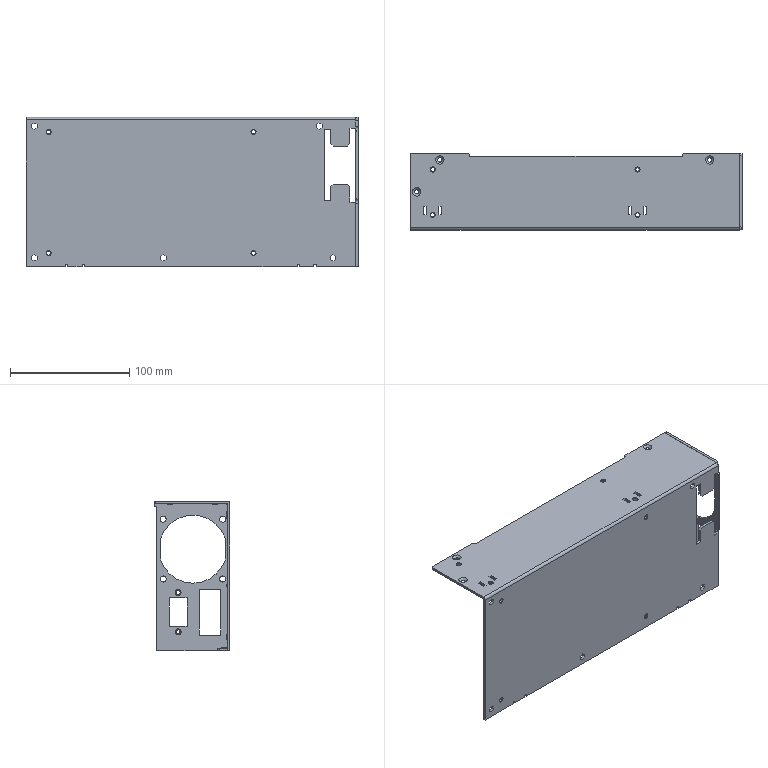Part | NX | features BREP 1 | 1 solid | 208 faces | box 278 x 63.5 x 125 mm | volume 107480 mm3 | plane 127 | cylinder 54 | torus 24 | cone 3 | commonest cylinder face diameters 2 x16 3.3 x10 4 x9 4.3 x4 5.1 x4 3.5 x3